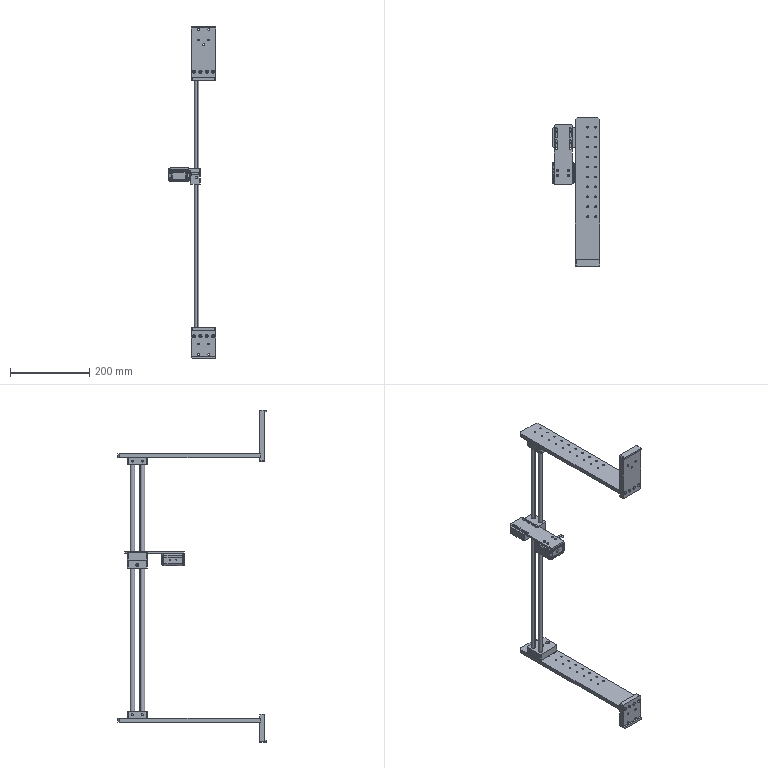Part | SolidWorks | 33 solids | 3178 faces | volume 984794 mm3 | cylinder 1212 | plane 1013 | spline 492 | cone 234 | torus 169 | sphere 58 | commonest cylinder face diameters 1.713 x174 1.376 x124 4 x107 4.2 x100 8 x70 1 x68